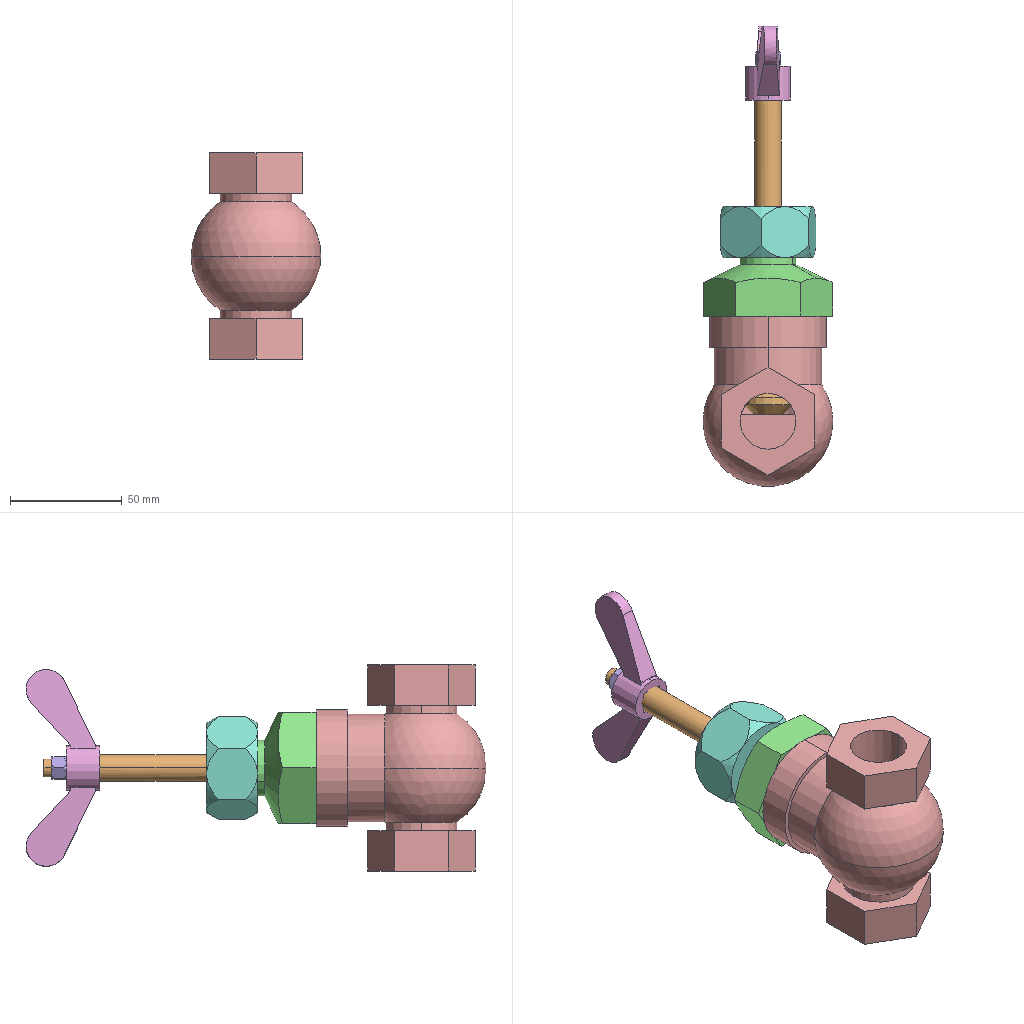Assembly | SolidWorks | 8 different items | 8 placed | box 58 x 205 x 92 mm
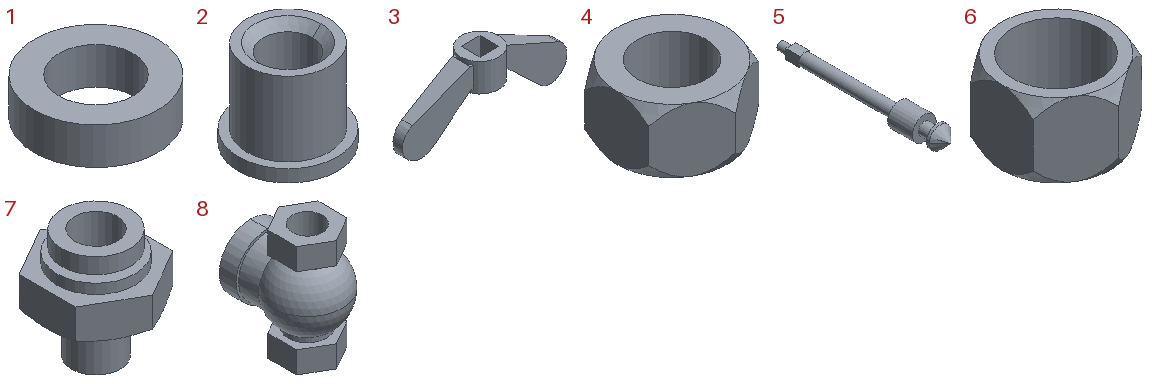Parts list (item | quantity | size | volume | features):
1 | x1 | 20 x 20 x 6 mm | 1206 mm3 | features Extrusion 1
2 | x1 | 24 x 24 x 21 mm | 4553 mm3 | features ICE 2, Chamfer 1, Extrusion 1
3 | x1 | 88 x 20 x 33 mm | 11211 mm3 | features ICE 2, Extrusion 1, MirrorPattern 1
4 | x1 | 40 x 46.188 x 23 mm | 22052 mm3 | features ICE 3, Extrusion 1, MirrorPattern 1
5 | x1 | 24 x 172 x 24 mm | 28435 mm3 | features ICE 2, Revolution 1
6 | x1 | 10 x 11.547 x 6.8 mm | 240.578 mm3 | features ICE 2, Extrusion 1, MirrorPattern 1
7 | x1 | 50 x 57.735 x 56 mm | 48059 mm3 | features ICE 6, Extrusion 1, RevCut 1
8 | x1 | 58 x 76 x 92 mm | 132810 mm3 | features ICE 8, RevCut 3, MirrorPattern 1, Revolution 1
Mates (type | each side: item.copy, entity, surface, feature):
Concentric | 8.1 face cylinder Cut-Extrude2 | 7.1 face cylinder Boss-Extrude5
Coincident | 8.1 face plane Boss-Extrude1 | 7.1 face plane Boss-Extrude1
Parallel | 8.1 face plane Mirror1 | 7.1 face plane Boss-Extrude1
Concentric | 5.1 face cylinder Revolve1 | 7.1 face cylinder Cut-Extrude2
Coincident | 8.1 face cone Cut-Revolve1 | 5.1 face cone Revolve1
Concentric | 1.1 face cylinder Boss-Extrude1 | 5.1 face cylinder Revolve1
Concentric | 4.1 face cylinder Cut-Extrude3 | 5.1 face cylinder Revolve1
Coincident | 1.1 face plane Boss-Extrude1 | 5.1 face plane Revolve1
Concentric | 1.1 face cylinder Boss-Extrude1 | 7.1 face cylinder Cut-Extrude1
Concentric | 2.1 face cylinder Boss-Extrude2 | 7.1 face cylinder Boss-Extrude2
Coincident | 2.1 face plane Boss-Extrude1 | 7.1 face plane Boss-Extrude2
Coincident | 2.1 face plane Boss-Extrude1 | 4.1 face plane Cut-Extrude2
Concentric | 3.1 face cylinder Boss-Extrude1 | 5.1 face cylinder Revolve1
Parallel | 3.1 edge | 5.1 edge
Concentric | 5.1 face cylinder Boss-Extrude2 | 6.1 face cylinder Cut-Extrude3
Coincident | 3.1 face plane Boss-Extrude1 | 5.1 face plane Boss-Extrude1
Coincident | 3.1 face plane Boss-Extrude1 | 6.1 face plane Boss-Extrude1